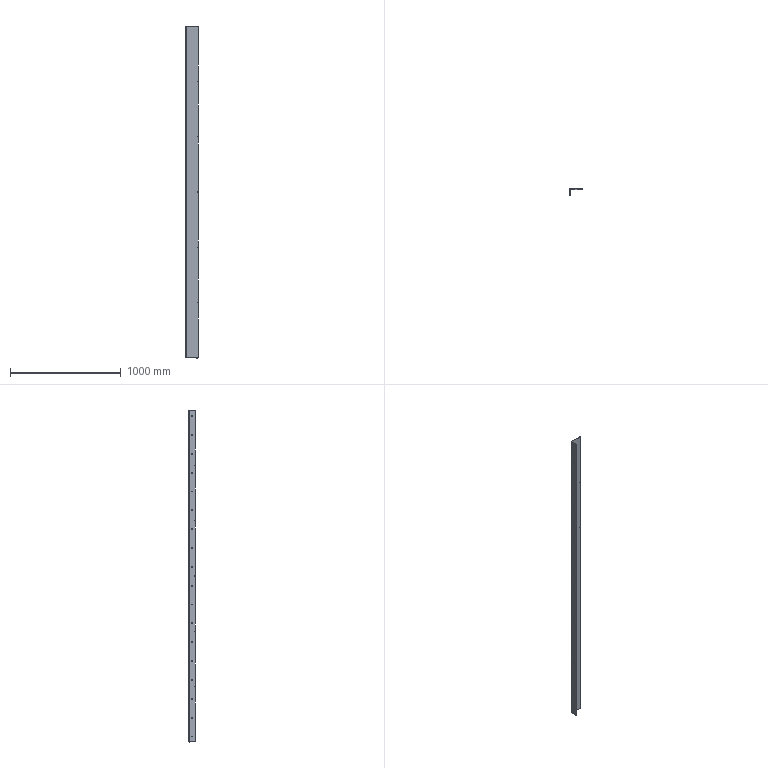Part | STEP file | TS-003-01 | 1 solid | 98 faces | box 109.914 x 59.871 x 2995 mm | volume 1488875 mm3 | plane 60 | cylinder 38 | commonest cylinder face diameters 8 x36 0.4 x1 6.4 x1